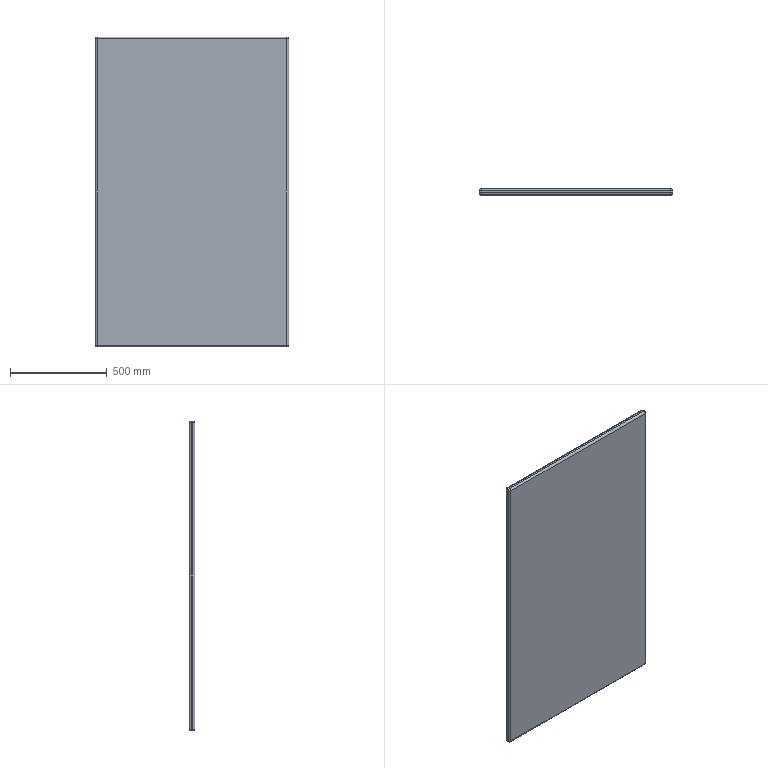Part | SolidWorks | features Extrusion 1, Fillet 1 | 1 solid | 26 faces | box 1000 x 30 x 1600 mm | volume 47775578 mm3 | cylinder 12 | sphere 8 | plane 6 | commonest cylinder face diameters 20 x12
STEP:
#1=CARTESIAN_POINT('',(500.,20.,-790.));
#2=VERTEX_POINT('',#1);
#3=CARTESIAN_POINT('',(500.,20.,790.));
#4=VERTEX_POINT('',#3);
#5=CARTESIAN_POINT('',(500.,20.,800.));
#6=DIRECTION('',(0.,0.,1.));
#7=VECTOR('',#6,1000.);
#8=LINE('',#5,#7);
#9=EDGE_CURVE('',#2,#4,#8,.T.);
#10=ORIENTED_EDGE('',*,*,#9,.T.);
#11=CARTESIAN_POINT('',(500.,10.,790.));
#12=VERTEX_POINT('',#11);
#13=CARTESIAN_POINT('',(500.,30.,790.));
#14=DIRECTION('',(0.,-1.,0.));
#15=VECTOR('',#14,1000.);
#16=LINE('',#13,#15);
#17=EDGE_CURVE('',#4,#12,#16,.T.);
#18=ORIENTED_EDGE('',*,*,#17,.T.);
#19=CARTESIAN_POINT('',(500.,10.,-790.));
#20=VERTEX_POINT('',#19);
#21=CARTESIAN_POINT('',(500.,10.,-800.));
#22=DIRECTION('',(0.,0.,-1.));
#23=VECTOR('',#22,1000.);
#24=LINE('',#21,#23);
#25=EDGE_CURVE('',#12,#20,#24,.T.);
#26=ORIENTED_EDGE('',*,*,#25,.T.);
#27=CARTESIAN_POINT('',(500.,30.,-790.));
#28=DIRECTION('',(0.,1.,0.));
#29=VECTOR('',#28,1000.);
#30=LINE('',#27,#29);
#31=EDGE_CURVE('',#20,#2,#30,.T.);
#32=ORIENTED_EDGE('',*,*,#31,.T.);
#33=EDGE_LOOP('',(#10,#18,#26,#32));
#34=FACE_OUTER_BOUND('',#33,.T.);
#35=CARTESIAN_POINT('',(500.,30.,-800.));
#36=DIRECTION('',(-1.,0.,0.));
#37=DIRECTION('',(0.,0.,1.));
#38=AXIS2_PLACEMENT_3D('',#35,#36,#37);
#39=PLANE('',#38);
#40=ADVANCED_FACE('',(#34),#39,.F.);
#41=CARTESIAN_POINT('',(-490.,10.,-800.));
#42=VERTEX_POINT('',#41);
#43=CARTESIAN_POINT('',(-490.,20.,-800.));
#44=VERTEX_POINT('',#43);
#45=CARTESIAN_POINT('',(-490.,30.,-800.));
#46=DIRECTION('',(0.,1.,0.));
#47=VECTOR('',#46,1000.);
#48=LINE('',#45,#47);
#49=EDGE_CURVE('',#42,#44,#48,.T.);
#50=ORIENTED_EDGE('',*,*,#49,.T.);
#51=CARTESIAN_POINT('',(490.,20.,-800.));
#52=VERTEX_POINT('',#51);
#53=CARTESIAN_POINT('',(500.,20.,-800.));
#54=DIRECTION('',(1.,0.,0.));
#55=VECTOR('',#54,1000.);
#56=LINE('',#53,#55);
#57=EDGE_CURVE('',#44,#52,#56,.T.);
#58=ORIENTED_EDGE('',*,*,#57,.T.);
#59=CARTESIAN_POINT('',(490.,10.,-800.));
#60=VERTEX_POINT('',#59);
#61=CARTESIAN_POINT('',(490.,30.,-800.));
#62=DIRECTION('',(0.,-1.,0.));
#63=VECTOR('',#62,1000.);
#64=LINE('',#61,#63);
#65=EDGE_CURVE('',#52,#60,#64,.T.);
#66=ORIENTED_EDGE('',*,*,#65,.T.);
#67=CARTESIAN_POINT('',(-500.,10.,-800.));
#68=DIRECTION('',(-1.,0.,0.));
#69=VECTOR('',#68,1000.);
#70=LINE('',#67,#69);
#71=EDGE_CURVE('',#60,#42,#70,.T.);
#72=ORIENTED_EDGE('',*,*,#71,.T.);
#73=EDGE_LOOP('',(#50,#58,#66,#72));
#74=FACE_OUTER_BOUND('',#73,.T.);
#75=CARTESIAN_POINT('',(-500.,30.,-800.));
#76=DIRECTION('',(0.,0.,1.));
#77=DIRECTION('',(1.,0.,0.));
#78=AXIS2_PLACEMENT_3D('',#75,#76,#77);
#79=PLANE('',#78);
#80=ADVANCED_FACE('',(#74),#79,.F.);
#81=CARTESIAN_POINT('',(-500.,20.,790.));
#82=VERTEX_POINT('',#81);
#83=CARTESIAN_POINT('',(-500.,20.,-790.));
#84=VERTEX_POINT('',#83);
#85=CARTESIAN_POINT('',(-500.,20.,-800.));
#86=DIRECTION('',(0.,0.,-1.));
#87=VECTOR('',#86,1000.);
#88=LINE('',#85,#87);
#89=EDGE_CURVE('',#82,#84,#88,.T.);
#90=ORIENTED_EDGE('',*,*,#89,.T.);
#91=CARTESIAN_POINT('',(-500.,10.,-790.));
#92=VERTEX_POINT('',#91);
#93=CARTESIAN_POINT('',(-500.,30.,-790.));
#94=DIRECTION('',(0.,-1.,0.));
#95=VECTOR('',#94,1000.);
#96=LINE('',#93,#95);
#97=EDGE_CURVE('',#84,#92,#96,.T.);
#98=ORIENTED_EDGE('',*,*,#97,.T.);
#99=CARTESIAN_POINT('',(-500.,10.,790.));
#100=VERTEX_POINT('',#99);
#101=CARTESIAN_POINT('',(-500.,10.,-800.));
#102=DIRECTION('',(0.,0.,1.));
#103=VECTOR('',#102,1000.);
#104=LINE('',#101,#103);
#105=EDGE_CURVE('',#92,#100,#104,.T.);
#106=ORIENTED_EDGE('',*,*,#105,.T.);
#107=CARTESIAN_POINT('',(-500.,30.,790.));
#108=DIRECTION('',(0.,1.,0.));
#109=VECTOR('',#108,1000.);
#110=LINE('',#107,#109);
#111=EDGE_CURVE('',#100,#82,#110,.T.);
#112=ORIENTED_EDGE('',*,*,#111,.T.);
#113=EDGE_LOOP('',(#90,#98,#106,#112));
#114=FACE_OUTER_BOUND('',#113,.T.);
#115=CARTESIAN_POINT('',(-500.,30.,-800.));
#116=DIRECTION('',(1.,0.,0.));
#117=DIRECTION('',(0.,0.,-1.));
#118=AXIS2_PLACEMENT_3D('',#115,#116,#117);
#119=PLANE('',#118);
#120=ADVANCED_FACE('',(#114),#119,.F.);
#121=CARTESIAN_POINT('',(490.,20.,800.));
#122=VERTEX_POINT('',#121);
#123=CARTESIAN_POINT('',(-490.,20.,800.));
#124=VERTEX_POINT('',#123);
#125=CARTESIAN_POINT('',(-500.,20.,800.));
#126=DIRECTION('',(-1.,0.,0.));
#127=VECTOR('',#126,1000.);
#128=LINE('',#125,#127);
#129=EDGE_CURVE('',#122,#124,#128,.T.);
#130=ORIENTED_EDGE('',*,*,#129,.T.);
#131=CARTESIAN_POINT('',(-490.,10.,800.));
#132=VERTEX_POINT('',#131);
#133=CARTESIAN_POINT('',(-490.,30.,800.));
#134=DIRECTION('',(0.,-1.,0.));
#135=VECTOR('',#134,1000.);
#136=LINE('',#133,#135);
#137=EDGE_CURVE('',#124,#132,#136,.T.);
#138=ORIENTED_EDGE('',*,*,#137,.T.);
#139=CARTESIAN_POINT('',(490.,10.,800.));
#140=VERTEX_POINT('',#139);
#141=CARTESIAN_POINT('',(-500.,10.,800.));
#142=DIRECTION('',(1.,0.,0.));
#143=VECTOR('',#142,1000.);
#144=LINE('',#141,#143);
#145=EDGE_CURVE('',#132,#140,#144,.T.);
#146=ORIENTED_EDGE('',*,*,#145,.T.);
#147=CARTESIAN_POINT('',(490.,30.,800.));
#148=DIRECTION('',(0.,1.,0.));
#149=VECTOR('',#148,1000.);
#150=LINE('',#147,#149);
#151=EDGE_CURVE('',#140,#122,#150,.T.);
#152=ORIENTED_EDGE('',*,*,#151,.T.);
#153=EDGE_LOOP('',(#130,#138,#146,#152));
#154=FACE_OUTER_BOUND('',#153,.T.);
#155=CARTESIAN_POINT('',(-500.,30.,800.));
#156=DIRECTION('',(0.,0.,-1.));
#157=DIRECTION('',(-1.,0.,0.));
#158=AXIS2_PLACEMENT_3D('',#155,#156,#157);
#159=PLANE('',#158);
#160=ADVANCED_FACE('',(#154),#159,.F.);
#161=CARTESIAN_POINT('',(490.,30.,-790.));
#162=VERTEX_POINT('',#161);
#163=CARTESIAN_POINT('',(-490.,30.,-790.));
#164=VERTEX_POINT('',#163);
#165=CARTESIAN_POINT('',(-500.,30.,-790.));
#166=DIRECTION('',(-1.,0.,0.));
#167=VECTOR('',#166,1000.);
#168=LINE('',#165,#167);
#169=EDGE_CURVE('',#162,#164,#168,.T.);
#170=ORIENTED_EDGE('',*,*,#169,.T.);
#171=CARTESIAN_POINT('',(-490.,30.,790.));
#172=VERTEX_POINT('',#171);
#173=CARTESIAN_POINT('',(-490.,30.,800.));
#174=DIRECTION('',(0.,0.,1.));
#175=VECTOR('',#174,1000.);
#176=LINE('',#173,#175);
#177=EDGE_CURVE('',#164,#172,#176,.T.);
#178=ORIENTED_EDGE('',*,*,#177,.T.);
#179=CARTESIAN_POINT('',(490.,30.,790.));
#180=VERTEX_POINT('',#179);
#181=CARTESIAN_POINT('',(500.,30.,790.));
#182=DIRECTION('',(1.,0.,0.));
#183=VECTOR('',#182,1000.);
#184=LINE('',#181,#183);
#185=EDGE_CURVE('',#172,#180,#184,.T.);
#186=ORIENTED_EDGE('',*,*,#185,.T.);
#187=CARTESIAN_POINT('',(490.,30.,-800.));
#188=DIRECTION('',(0.,0.,-1.));
#189=VECTOR('',#188,1000.);
#190=LINE('',#187,#189);
#191=EDGE_CURVE('',#180,#162,#190,.T.);
#192=ORIENTED_EDGE('',*,*,#191,.T.);
#193=EDGE_LOOP('',(#170,#178,#186,#192));
#194=FACE_OUTER_BOUND('',#193,.T.);
#195=CARTESIAN_POINT('',(0.,30.,0.));
#196=DIRECTION('',(0.,1.,0.));
#197=DIRECTION('',(0.,0.,1.));
#198=AXIS2_PLACEMENT_3D('',#195,#196,#197);
#199=PLANE('',#198);
#200=ADVANCED_FACE('',(#194),#199,.T.);
#201=CARTESIAN_POINT('',(490.,0.,790.));
#202=VERTEX_POINT('',#201);
#203=CARTESIAN_POINT('',(-490.,0.,790.));
#204=VERTEX_POINT('',#203);
#205=CARTESIAN_POINT('',(0.,0.,790.));
#206=DIRECTION('',(-1.,0.,0.));
#207=VECTOR('',#206,1000.);
#208=LINE('',#205,#207);
#209=EDGE_CURVE('',#202,#204,#208,.T.);
#210=ORIENTED_EDGE('',*,*,#209,.T.);
#211=CARTESIAN_POINT('',(-490.,0.,-790.));
#212=VERTEX_POINT('',#211);
#213=CARTESIAN_POINT('',(-490.,0.,0.));
#214=DIRECTION('',(0.,0.,-1.));
#215=VECTOR('',#214,1000.);
#216=LINE('',#213,#215);
#217=EDGE_CURVE('',#204,#212,#216,.T.);
#218=ORIENTED_EDGE('',*,*,#217,.T.);
#219=CARTESIAN_POINT('',(490.,0.,-790.));
#220=VERTEX_POINT('',#219);
#221=CARTESIAN_POINT('',(0.,0.,-790.));
#222=DIRECTION('',(1.,0.,0.));
#223=VECTOR('',#222,1000.);
#224=LINE('',#221,#223);
#225=EDGE_CURVE('',#212,#220,#224,.T.);
#226=ORIENTED_EDGE('',*,*,#225,.T.);
#227=CARTESIAN_POINT('',(490.,0.,0.));
#228=DIRECTION('',(0.,0.,1.));
#229=VECTOR('',#228,1000.);
#230=LINE('',#227,#229);
#231=EDGE_CURVE('',#220,#202,#230,.T.);
#232=ORIENTED_EDGE('',*,*,#231,.T.);
#233=EDGE_LOOP('',(#210,#218,#226,#232));
#234=FACE_OUTER_BOUND('',#233,.T.);
#235=CARTESIAN_POINT('',(0.,0.,0.));
#236=DIRECTION('',(0.,1.,0.));
#237=DIRECTION('',(0.,0.,1.));
#238=AXIS2_PLACEMENT_3D('',#235,#236,#237);
#239=PLANE('',#238);
#240=ADVANCED_FACE('',(#234),#239,.F.);
#241=CARTESIAN_POINT('',(490.,10.,-790.));
#242=DIRECTION('',(0.,0.,-1.));
#243=DIRECTION('',(-1.,0.,0.));
#244=AXIS2_PLACEMENT_3D('',#241,#242,#243);
#245=CIRCLE('',#244,10.);
#246=EDGE_CURVE('',#20,#220,#245,.T.);
#247=ORIENTED_EDGE('',*,*,#246,.F.);
#248=ORIENTED_EDGE('',*,*,#25,.F.);
#249=CARTESIAN_POINT('',(490.,10.,790.));
#250=DIRECTION('',(0.,0.,1.));
#251=DIRECTION('',(1.,0.,0.));
#252=AXIS2_PLACEMENT_3D('',#249,#250,#251);
#253=CIRCLE('',#252,10.);
#254=EDGE_CURVE('',#202,#12,#253,.T.);
#255=ORIENTED_EDGE('',*,*,#254,.F.);
#256=ORIENTED_EDGE('',*,*,#231,.F.);
#257=EDGE_LOOP('',(#247,#248,#255,#256));
#258=FACE_OUTER_BOUND('',#257,.T.);
#259=CARTESIAN_POINT('',(490.,10.,-800.));
#260=DIRECTION('',(0.,0.,-1.));
#261=DIRECTION('',(-1.,0.,0.));
#262=AXIS2_PLACEMENT_3D('',#259,#260,#261);
#263=CYLINDRICAL_SURFACE('',#262,10.);
#264=ADVANCED_FACE('',(#258),#263,.T.);
#265=CARTESIAN_POINT('',(490.,10.,-790.));
#266=DIRECTION('',(0.,1.,0.));
#267=DIRECTION('',(0.,0.,-1.));
#268=AXIS2_PLACEMENT_3D('',#265,#266,#267);
#269=CIRCLE('',#268,10.);
#270=EDGE_CURVE('',#20,#60,#269,.T.);
#271=ORIENTED_EDGE('',*,*,#270,.F.);
#272=ORIENTED_EDGE('',*,*,#246,.T.);
#273=CARTESIAN_POINT('',(490.,10.,-790.));
#274=DIRECTION('',(-1.,0.,0.));
#275=DIRECTION('',(0.,0.,-1.));
#276=AXIS2_PLACEMENT_3D('',#273,#274,#275);
#277=CIRCLE('',#276,10.);
#278=EDGE_CURVE('',#60,#220,#277,.T.);
#279=ORIENTED_EDGE('',*,*,#278,.F.);
#280=EDGE_LOOP('',(#271,#272,#279));
#281=FACE_OUTER_BOUND('',#280,.T.);
#282=CARTESIAN_POINT('',(490.,10.,-790.));
#283=DIRECTION('',(0.,1.,0.));
#284=DIRECTION('',(1.,0.,0.));
#285=AXIS2_PLACEMENT_3D('',#282,#283,#284);
#286=SPHERICAL_SURFACE('',#285,10.);
#287=ADVANCED_FACE('',(#281),#286,.T.);
#288=CARTESIAN_POINT('',(490.,10.,790.));
#289=DIRECTION('',(-1.,0.,0.));
#290=DIRECTION('',(0.,0.,-1.));
#291=AXIS2_PLACEMENT_3D('',#288,#289,#290);
#292=CIRCLE('',#291,10.);
#293=EDGE_CURVE('',#202,#140,#292,.T.);
#294=ORIENTED_EDGE('',*,*,#293,.F.);
#295=ORIENTED_EDGE('',*,*,#254,.T.);
#296=CARTESIAN_POINT('',(490.,10.,790.));
#297=DIRECTION('',(0.,1.,0.));
#298=DIRECTION('',(0.,0.,-1.));
#299=AXIS2_PLACEMENT_3D('',#296,#297,#298);
#300=CIRCLE('',#299,10.);
#301=EDGE_CURVE('',#140,#12,#300,.T.);
#302=ORIENTED_EDGE('',*,*,#301,.F.);
#303=EDGE_LOOP('',(#294,#295,#302));
#304=FACE_OUTER_BOUND('',#303,.T.);
#305=CARTESIAN_POINT('',(490.,10.,790.));
#306=DIRECTION('',(0.,1.,0.));
#307=DIRECTION('',(1.,0.,0.));
#308=AXIS2_PLACEMENT_3D('',#305,#306,#307);
#309=SPHERICAL_SURFACE('',#308,10.);
#310=ADVANCED_FACE('',(#304),#309,.T.);
#311=ORIENTED_EDGE('',*,*,#278,.T.);
#312=ORIENTED_EDGE('',*,*,#225,.F.);
#313=CARTESIAN_POINT('',(-490.,10.,-790.));
#314=DIRECTION('',(-1.,0.,0.));
#315=DIRECTION('',(0.,0.,1.));
#316=AXIS2_PLACEMENT_3D('',#313,#314,#315);
#317=CIRCLE('',#316,10.);
#318=EDGE_CURVE('',#42,#212,#317,.T.);
#319=ORIENTED_EDGE('',*,*,#318,.F.);
#320=ORIENTED_EDGE('',*,*,#71,.F.);
#321=EDGE_LOOP('',(#311,#312,#319,#320));
#322=FACE_OUTER_BOUND('',#321,.T.);
#323=CARTESIAN_POINT('',(-500.,10.,-790.));
#324=DIRECTION('',(-1.,0.,0.));
#325=DIRECTION('',(0.,0.,1.));
#326=AXIS2_PLACEMENT_3D('',#323,#324,#325);
#327=CYLINDRICAL_SURFACE('',#326,10.);
#328=ADVANCED_FACE('',(#322),#327,.T.);
#329=ORIENTED_EDGE('',*,*,#270,.T.);
#330=ORIENTED_EDGE('',*,*,#65,.F.);
#331=CARTESIAN_POINT('',(490.,20.,-790.));
#332=DIRECTION('',(0.,1.,0.));
#333=DIRECTION('',(0.,0.,1.));
#334=AXIS2_PLACEMENT_3D('',#331,#332,#333);
#335=CIRCLE('',#334,10.);
#336=EDGE_CURVE('',#2,#52,#335,.T.);
#337=ORIENTED_EDGE('',*,*,#336,.F.);
#338=ORIENTED_EDGE('',*,*,#31,.F.);
#339=EDGE_LOOP('',(#329,#330,#337,#338));
#340=FACE_OUTER_BOUND('',#339,.T.);
#341=CARTESIAN_POINT('',(490.,30.,-790.));
#342=DIRECTION('',(0.,-1.,0.));
#343=DIRECTION('',(0.,0.,-1.));
#344=AXIS2_PLACEMENT_3D('',#341,#342,#343);
#345=CYLINDRICAL_SURFACE('',#344,10.);
#346=ADVANCED_FACE('',(#340),#345,.T.);
#347=CARTESIAN_POINT('',(490.,20.,790.));
#348=DIRECTION('',(0.,0.,1.));
#349=DIRECTION('',(1.,0.,0.));
#350=AXIS2_PLACEMENT_3D('',#347,#348,#349);
#351=CIRCLE('',#350,10.);
#352=EDGE_CURVE('',#4,#180,#351,.T.);
#353=ORIENTED_EDGE('',*,*,#352,.F.);
#354=ORIENTED_EDGE('',*,*,#9,.F.);
#355=CARTESIAN_POINT('',(490.,20.,-790.));
#356=DIRECTION('',(0.,0.,-1.));
#357=DIRECTION('',(-1.,0.,0.));
#358=AXIS2_PLACEMENT_3D('',#355,#356,#357);
#359=CIRCLE('',#358,10.);
#360=EDGE_CURVE('',#162,#2,#359,.T.);
#361=ORIENTED_EDGE('',*,*,#360,.F.);
#362=ORIENTED_EDGE('',*,*,#191,.F.);
#363=EDGE_LOOP('',(#353,#354,#361,#362));
#364=FACE_OUTER_BOUND('',#363,.T.);
#365=CARTESIAN_POINT('',(490.,20.,0.));
#366=DIRECTION('',(0.,0.,1.));
#367=DIRECTION('',(1.,0.,0.));
#368=AXIS2_PLACEMENT_3D('',#365,#366,#367);
#369=CYLINDRICAL_SURFACE('',#368,10.);
#370=ADVANCED_FACE('',(#364),#369,.T.);
#371=ORIENTED_EDGE('',*,*,#301,.T.);
#372=ORIENTED_EDGE('',*,*,#17,.F.);
#373=CARTESIAN_POINT('',(490.,20.,790.));
#374=DIRECTION('',(0.,1.,0.));
#375=DIRECTION('',(0.,0.,1.));
#376=AXIS2_PLACEMENT_3D('',#373,#374,#375);
#377=CIRCLE('',#376,10.);
#378=EDGE_CURVE('',#122,#4,#377,.T.);
#379=ORIENTED_EDGE('',*,*,#378,.F.);
#380=ORIENTED_EDGE('',*,*,#151,.F.);
#381=EDGE_LOOP('',(#371,#372,#379,#380));
#382=FACE_OUTER_BOUND('',#381,.T.);
#383=CARTESIAN_POINT('',(490.,30.,790.));
#384=DIRECTION('',(0.,-1.,0.));
#385=DIRECTION('',(0.,0.,-1.));
#386=AXIS2_PLACEMENT_3D('',#383,#384,#385);
#387=CYLINDRICAL_SURFACE('',#386,10.);
#388=ADVANCED_FACE('',(#382),#387,.T.);
#389=ORIENTED_EDGE('',*,*,#293,.T.);
#390=ORIENTED_EDGE('',*,*,#145,.F.);
#391=CARTESIAN_POINT('',(-490.,10.,790.));
#392=DIRECTION('',(-1.,0.,0.));
#393=DIRECTION('',(0.,0.,1.));
#394=AXIS2_PLACEMENT_3D('',#391,#392,#393);
#395=CIRCLE('',#394,10.);
#396=EDGE_CURVE('',#204,#132,#395,.T.);
#397=ORIENTED_EDGE('',*,*,#396,.F.);
#398=ORIENTED_EDGE('',*,*,#209,.F.);
#399=EDGE_LOOP('',(#389,#390,#397,#398));
#400=FACE_OUTER_BOUND('',#399,.T.);
#401=CARTESIAN_POINT('',(-500.,10.,790.));
#402=DIRECTION('',(1.,0.,0.));
#403=DIRECTION('',(0.,0.,-1.));
#404=AXIS2_PLACEMENT_3D('',#401,#402,#403);
#405=CYLINDRICAL_SURFACE('',#404,10.);
#406=ADVANCED_FACE('',(#400),#405,.T.);
#407=CARTESIAN_POINT('',(-490.,10.,-790.));
#408=DIRECTION('',(0.,0.,-1.));
#409=DIRECTION('',(-1.,0.,0.));
#410=AXIS2_PLACEMENT_3D('',#407,#408,#409);
#411=CIRCLE('',#410,10.);
#412=EDGE_CURVE('',#212,#92,#411,.T.);
#413=ORIENTED_EDGE('',*,*,#412,.F.);
#414=ORIENTED_EDGE('',*,*,#217,.F.);
#415=CARTESIAN_POINT('',(-490.,10.,790.));
#416=DIRECTION('',(0.,0.,1.));
#417=DIRECTION('',(1.,0.,0.));
#418=AXIS2_PLACEMENT_3D('',#415,#416,#417);
#419=CIRCLE('',#418,10.);
#420=EDGE_CURVE('',#100,#204,#419,.T.);
#421=ORIENTED_EDGE('',*,*,#420,.F.);
#422=ORIENTED_EDGE('',*,*,#105,.F.);
#423=EDGE_LOOP('',(#413,#414,#421,#422));
#424=FACE_OUTER_BOUND('',#423,.T.);
#425=CARTESIAN_POINT('',(-490.,10.,-800.));
#426=DIRECTION('',(0.,0.,1.));
#427=DIRECTION('',(1.,0.,0.));
#428=AXIS2_PLACEMENT_3D('',#425,#426,#427);
#429=CYLINDRICAL_SURFACE('',#428,10.);
#430=ADVANCED_FACE('',(#424),#429,.T.);
#431=ORIENTED_EDGE('',*,*,#318,.T.);
#432=ORIENTED_EDGE('',*,*,#412,.T.);
#433=CARTESIAN_POINT('',(-490.,10.,-790.));
#434=DIRECTION('',(0.,1.,0.));
#435=DIRECTION('',(0.,0.,-1.));
#436=AXIS2_PLACEMENT_3D('',#433,#434,#435);
#437=CIRCLE('',#436,10.);
#438=EDGE_CURVE('',#42,#92,#437,.T.);
#439=ORIENTED_EDGE('',*,*,#438,.F.);
#440=EDGE_LOOP('',(#431,#432,#439));
#441=FACE_OUTER_BOUND('',#440,.T.);
#442=CARTESIAN_POINT('',(-490.,10.,-790.));
#443=DIRECTION('',(0.,1.,0.));
#444=DIRECTION('',(1.,0.,0.));
#445=AXIS2_PLACEMENT_3D('',#442,#443,#444);
#446=SPHERICAL_SURFACE('',#445,10.);
#447=ADVANCED_FACE('',(#441),#446,.T.);
#448=ORIENTED_EDGE('',*,*,#360,.T.);
#449=ORIENTED_EDGE('',*,*,#336,.T.);
#450=CARTESIAN_POINT('',(490.,20.,-790.));
#451=DIRECTION('',(-1.,0.,0.));
#452=DIRECTION('',(0.,0.,-1.));
#453=AXIS2_PLACEMENT_3D('',#450,#451,#452);
#454=CIRCLE('',#453,10.);
#455=EDGE_CURVE('',#162,#52,#454,.T.);
#456=ORIENTED_EDGE('',*,*,#455,.F.);
#457=EDGE_LOOP('',(#448,#449,#456));
#458=FACE_OUTER_BOUND('',#457,.T.);
#459=CARTESIAN_POINT('',(490.,20.,-790.));
#460=DIRECTION('',(0.,1.,0.));
#461=DIRECTION('',(1.,0.,0.));
#462=AXIS2_PLACEMENT_3D('',#459,#460,#461);
#463=SPHERICAL_SURFACE('',#462,10.);
#464=ADVANCED_FACE('',(#458),#463,.T.);
#465=ORIENTED_EDGE('',*,*,#378,.T.);
#466=ORIENTED_EDGE('',*,*,#352,.T.);
#467=CARTESIAN_POINT('',(490.,20.,790.));
#468=DIRECTION('',(-1.,0.,0.));
#469=DIRECTION('',(0.,0.,-1.));
#470=AXIS2_PLACEMENT_3D('',#467,#468,#469);
#471=CIRCLE('',#470,10.);
#472=EDGE_CURVE('',#122,#180,#471,.T.);
#473=ORIENTED_EDGE('',*,*,#472,.F.);
#474=EDGE_LOOP('',(#465,#466,#473));
#475=FACE_OUTER_BOUND('',#474,.T.);
#476=CARTESIAN_POINT('',(490.,20.,790.));
#477=DIRECTION('',(0.,1.,0.));
#478=DIRECTION('',(1.,0.,0.));
#479=AXIS2_PLACEMENT_3D('',#476,#477,#478);
#480=SPHERICAL_SURFACE('',#479,10.);
#481=ADVANCED_FACE('',(#475),#480,.T.);
#482=ORIENTED_EDGE('',*,*,#420,.T.);
#483=ORIENTED_EDGE('',*,*,#396,.T.);
#484=CARTESIAN_POINT('',(-490.,10.,790.));
#485=DIRECTION('',(0.,1.,0.));
#486=DIRECTION('',(0.,0.,-1.));
#487=AXIS2_PLACEMENT_3D('',#484,#485,#486);
#488=CIRCLE('',#487,10.);
#489=EDGE_CURVE('',#100,#132,#488,.T.);
#490=ORIENTED_EDGE('',*,*,#489,.F.);
#491=EDGE_LOOP('',(#482,#483,#490));
#492=FACE_OUTER_BOUND('',#491,.T.);
#493=CARTESIAN_POINT('',(-490.,10.,790.));
#494=DIRECTION('',(0.,1.,0.));
#495=DIRECTION('',(1.,0.,0.));
#496=AXIS2_PLACEMENT_3D('',#493,#494,#495);
#497=SPHERICAL_SURFACE('',#496,10.);
#498=ADVANCED_FACE('',(#492),#497,.T.);
#499=ORIENTED_EDGE('',*,*,#438,.T.);
#500=ORIENTED_EDGE('',*,*,#97,.F.);
#501=CARTESIAN_POINT('',(-490.,20.,-790.));
#502=DIRECTION('',(0.,1.,0.));
#503=DIRECTION('',(0.,0.,1.));
#504=AXIS2_PLACEMENT_3D('',#501,#502,#503);
#505=CIRCLE('',#504,10.);
#506=EDGE_CURVE('',#44,#84,#505,.T.);
#507=ORIENTED_EDGE('',*,*,#506,.F.);
#508=ORIENTED_EDGE('',*,*,#49,.F.);
#509=EDGE_LOOP('',(#499,#500,#507,#508));
#510=FACE_OUTER_BOUND('',#509,.T.);
#511=CARTESIAN_POINT('',(-490.,30.,-790.));
#512=DIRECTION('',(0.,-1.,0.));
#513=DIRECTION('',(0.,0.,-1.));
#514=AXIS2_PLACEMENT_3D('',#511,#512,#513);
#515=CYLINDRICAL_SURFACE('',#514,10.);
#516=ADVANCED_FACE('',(#510),#515,.T.);
#517=ORIENTED_EDGE('',*,*,#455,.T.);
#518=ORIENTED_EDGE('',*,*,#57,.F.);
#519=CARTESIAN_POINT('',(-490.,20.,-790.));
#520=DIRECTION('',(-1.,0.,0.));
#521=DIRECTION('',(0.,0.,1.));
#522=AXIS2_PLACEMENT_3D('',#519,#520,#521);
#523=CIRCLE('',#522,10.);
#524=EDGE_CURVE('',#164,#44,#523,.T.);
#525=ORIENTED_EDGE('',*,*,#524,.F.);
#526=ORIENTED_EDGE('',*,*,#169,.F.);
#527=EDGE_LOOP('',(#517,#518,#525,#526));
#528=FACE_OUTER_BOUND('',#527,.T.);
#529=CARTESIAN_POINT('',(0.,20.,-790.));
#530=DIRECTION('',(1.,0.,0.));
#531=DIRECTION('',(0.,0.,-1.));
#532=AXIS2_PLACEMENT_3D('',#529,#530,#531);
#533=CYLINDRICAL_SURFACE('',#532,10.);
#534=ADVANCED_FACE('',(#528),#533,.T.);
#535=ORIENTED_EDGE('',*,*,#472,.T.);
#536=ORIENTED_EDGE('',*,*,#185,.F.);
#537=CARTESIAN_POINT('',(-490.,20.,790.));
#538=DIRECTION('',(-1.,0.,0.));
#539=DIRECTION('',(0.,-1.,0.));
#540=AXIS2_PLACEMENT_3D('',#537,#538,#539);
#541=CIRCLE('',#540,10.);
#542=EDGE_CURVE('',#124,#172,#541,.T.);
#543=ORIENTED_EDGE('',*,*,#542,.F.);
#544=ORIENTED_EDGE('',*,*,#129,.F.);
#545=EDGE_LOOP('',(#535,#536,#543,#544));
#546=FACE_OUTER_BOUND('',#545,.T.);
#547=CARTESIAN_POINT('',(0.,20.,790.));
#548=DIRECTION('',(-1.,0.,0.));
#549=DIRECTION('',(0.,0.,1.));
#550=AXIS2_PLACEMENT_3D('',#547,#548,#549);
#551=CYLINDRICAL_SURFACE('',#550,10.);
#552=ADVANCED_FACE('',(#546),#551,.T.);
#553=ORIENTED_EDGE('',*,*,#489,.T.);
#554=ORIENTED_EDGE('',*,*,#137,.F.);
#555=CARTESIAN_POINT('',(-490.,20.,790.));
#556=DIRECTION('',(0.,1.,0.));
#557=DIRECTION('',(0.,0.,1.));
#558=AXIS2_PLACEMENT_3D('',#555,#556,#557);
#559=CIRCLE('',#558,10.);
#560=EDGE_CURVE('',#82,#124,#559,.T.);
#561=ORIENTED_EDGE('',*,*,#560,.F.);
#562=ORIENTED_EDGE('',*,*,#111,.F.);
#563=EDGE_LOOP('',(#553,#554,#561,#562));
#564=FACE_OUTER_BOUND('',#563,.T.);
#565=CARTESIAN_POINT('',(-490.,30.,790.));
#566=DIRECTION('',(0.,-1.,0.));
#567=DIRECTION('',(0.,0.,-1.));
#568=AXIS2_PLACEMENT_3D('',#565,#566,#567);
#569=CYLINDRICAL_SURFACE('',#568,10.);
#570=ADVANCED_FACE('',(#564),#569,.T.);
#571=ORIENTED_EDGE('',*,*,#524,.T.);
#572=ORIENTED_EDGE('',*,*,#506,.T.);
#573=CARTESIAN_POINT('',(-490.,20.,-790.));
#574=DIRECTION('',(0.,0.,1.));
#575=DIRECTION('',(-1.,0.,0.));
#576=AXIS2_PLACEMENT_3D('',#573,#574,#575);
#577=CIRCLE('',#576,10.);
#578=EDGE_CURVE('',#164,#84,#577,.T.);
#579=ORIENTED_EDGE('',*,*,#578,.F.);
#580=EDGE_LOOP('',(#571,#572,#579));
#581=FACE_OUTER_BOUND('',#580,.T.);
#582=CARTESIAN_POINT('',(-490.,20.,-790.));
#583=DIRECTION('',(0.,1.,0.));
#584=DIRECTION('',(1.,0.,0.));
#585=AXIS2_PLACEMENT_3D('',#582,#583,#584);
#586=SPHERICAL_SURFACE('',#585,10.);
#587=ADVANCED_FACE('',(#581),#586,.T.);
#588=ORIENTED_EDGE('',*,*,#560,.T.);
#589=ORIENTED_EDGE('',*,*,#542,.T.);
#590=CARTESIAN_POINT('',(-490.,20.,790.));
#591=DIRECTION('',(0.,0.,-1.));
#592=DIRECTION('',(1.,0.,0.));
#593=AXIS2_PLACEMENT_3D('',#590,#591,#592);
#594=CIRCLE('',#593,10.);
#595=EDGE_CURVE('',#82,#172,#594,.T.);
#596=ORIENTED_EDGE('',*,*,#595,.F.);
#597=EDGE_LOOP('',(#588,#589,#596));
#598=FACE_OUTER_BOUND('',#597,.T.);
#599=CARTESIAN_POINT('',(-490.,20.,790.));
#600=DIRECTION('',(0.,1.,0.));
#601=DIRECTION('',(1.,0.,0.));
#602=AXIS2_PLACEMENT_3D('',#599,#600,#601);
#603=SPHERICAL_SURFACE('',#602,10.);
#604=ADVANCED_FACE('',(#598),#603,.T.);
#605=ORIENTED_EDGE('',*,*,#578,.T.);
#606=ORIENTED_EDGE('',*,*,#89,.F.);
#607=ORIENTED_EDGE('',*,*,#595,.T.);
#608=ORIENTED_EDGE('',*,*,#177,.F.);
#609=EDGE_LOOP('',(#605,#606,#607,#608));
#610=FACE_OUTER_BOUND('',#609,.T.);
#611=CARTESIAN_POINT('',(-490.,20.,0.));
#612=DIRECTION('',(0.,0.,-1.));
#613=DIRECTION('',(-1.,0.,0.));
#614=AXIS2_PLACEMENT_3D('',#611,#612,#613);
#615=CYLINDRICAL_SURFACE('',#614,10.);
#616=ADVANCED_FACE('',(#610),#615,.T.);
#617=CLOSED_SHELL('',(#40,#80,#120,#160,#200,#240,#264,#287,#310,#328,#346,#370,#388,#406,#430,#447,#464,#481,#498,#516,#534,#552,#570,#587,#604,#616));
#618=MANIFOLD_SOLID_BREP('',#617);
#619=CARTESIAN_POINT('',(0.,0.,0.));
#620=DIRECTION('',(0.,0.,1.));
#621=DIRECTION('',(1.,0.,0.));
#622=AXIS2_PLACEMENT_3D('',#619,#620,#621);
#623=(LENGTH_UNIT()NAMED_UNIT(*)SI_UNIT(.MILLI.,.METRE.));
#624=UNCERTAINTY_MEASURE_WITH_UNIT(LENGTH_MEASURE(0.00001),#623,'','');
#625=(NAMED_UNIT(*)PLANE_ANGLE_UNIT()SI_UNIT($,.RADIAN.));
#626=(NAMED_UNIT(*)SI_UNIT($,.STERADIAN.)SOLID_ANGLE_UNIT());
#627=(GEOMETRIC_REPRESENTATION_CONTEXT(3)GLOBAL_UNCERTAINTY_ASSIGNED_CONTEXT((#624))GLOBAL_UNIT_ASSIGNED_CONTEXT((#623,#625,#626))REPRESENTATION_CONTEXT('',''));
#628=ADVANCED_BREP_SHAPE_REPRESENTATION('',(#618,#622),#627);